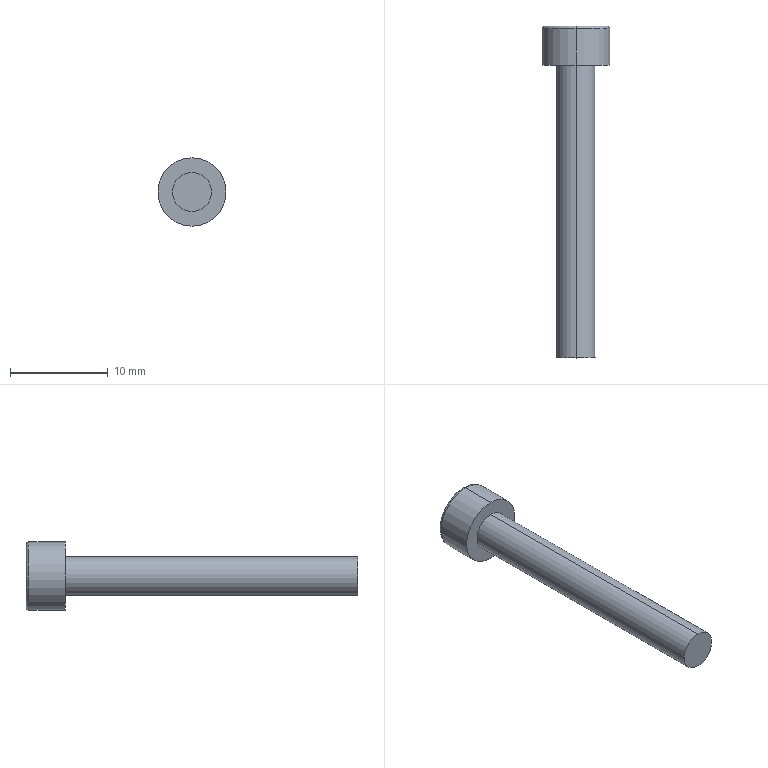Part | STEP file | M4 socket head cap screw simplified_M4X30 | 1 solid | 16 faces | box 7 x 34 x 7 mm | volume 513.868 mm3 | plane 10 | cylinder 4 | torus 2 | commonest cylinder face diameters 4 x2 7 x2
STEP:
#1=CARTESIAN_POINT('',(0.,0.,0.));
#2=DIRECTION('',(0.,0.,1.));
#3=DIRECTION('',(1.,0.,0.));
#4=AXIS2_PLACEMENT_3D('',#1,#2,#3);
#5=CARTESIAN_POINT('',(0.,0.,3.2));
#6=VERTEX_POINT('',#5);
#7=CARTESIAN_POINT('',(0.,0.,-3.2));
#8=VERTEX_POINT('',#7);
#9=CARTESIAN_POINT('',(0.,0.,0.));
#10=DIRECTION('',(0.,1.,0.));
#11=DIRECTION('',(0.,0.,-1.));
#12=AXIS2_PLACEMENT_3D('',#9,#10,#11);
#13=CIRCLE('',#12,3.2);
#14=CARTESIAN_POINT('',(0.,-0.3,0.));
#15=DIRECTION('',(0.,-1.,0.));
#16=DIRECTION('',(0.,0.,-1.));
#17=AXIS2_PLACEMENT_3D('',#14,#15,#16);
#18=TOROIDAL_SURFACE('',#17,3.2,0.3);
#19=CARTESIAN_POINT('',(6.283,4.712));
#20=DIRECTION('',(-1.,0.));
#21=VECTOR('',#20,1.);
#22=LINE('',#19,#21);
#23=(GEOMETRIC_REPRESENTATION_CONTEXT(2)PARAMETRIC_REPRESENTATION_CONTEXT()REPRESENTATION_CONTEXT('',''));
#24=DEFINITIONAL_REPRESENTATION('',(#22),#23);
#25=PCURVE('',#18,#24);
#26=CARTESIAN_POINT('',(0.,0.,0.));
#27=DIRECTION('',(0.,-1.,0.));
#28=DIRECTION('',(0.,0.,-1.));
#29=AXIS2_PLACEMENT_3D('',#26,#27,#28);
#30=PLANE('',#29);
#31=CARTESIAN_POINT('',(3.2,0.));
#32=CARTESIAN_POINT('',(3.2,-5.543));
#33=CARTESIAN_POINT('',(-1.6,-2.771));
#34=CARTESIAN_POINT('',(-6.4,0.));
#35=CARTESIAN_POINT('',(-1.6,2.771));
#36=CARTESIAN_POINT('',(3.2,5.543));
#37=CARTESIAN_POINT('',(3.2,0.));
#38=(BOUNDED_CURVE()B_SPLINE_CURVE(2,(#31,#32,#33,#34,#35,#36,#37),.UNSPECIFIED.,.T.,.F.)B_SPLINE_CURVE_WITH_KNOTS((1,2,2,2,2,1),(-2.094,0.,2.094,4.189,6.283,8.378),.UNSPECIFIED.)CURVE()GEOMETRIC_REPRESENTATION_ITEM()RATIONAL_B_SPLINE_CURVE((1.,0.5,1.,0.5,1.,0.5,1.))REPRESENTATION_ITEM(''));
#39=(GEOMETRIC_REPRESENTATION_CONTEXT(2)PARAMETRIC_REPRESENTATION_CONTEXT()REPRESENTATION_CONTEXT('',''));
#40=DEFINITIONAL_REPRESENTATION('',(#38),#39);
#41=PCURVE('',#30,#40);
#42=SURFACE_CURVE('',#13,(#25,#41),.PCURVE_S1.);
#43=EDGE_CURVE('',#6,#8,#42,.T.);
#44=ORIENTED_EDGE('',*,*,#43,.F.);
#45=CARTESIAN_POINT('',(0.,-0.3,3.5));
#46=VERTEX_POINT('',#45);
#47=CARTESIAN_POINT('',(0.,-0.3,3.2));
#48=DIRECTION('',(1.,0.,0.));
#49=DIRECTION('',(0.,0.,-1.));
#50=AXIS2_PLACEMENT_3D('',#47,#48,#49);
#51=CIRCLE('',#50,0.3);
#52=CARTESIAN_POINT('',(3.142,3.142));
#53=DIRECTION('',(0.,1.));
#54=VECTOR('',#53,1.);
#55=LINE('',#52,#54);
#56=(GEOMETRIC_REPRESENTATION_CONTEXT(2)PARAMETRIC_REPRESENTATION_CONTEXT()REPRESENTATION_CONTEXT('',''));
#57=DEFINITIONAL_REPRESENTATION('',(#55),#56);
#58=PCURVE('',#18,#57);
#59=CARTESIAN_POINT('',(0.,-0.3,0.));
#60=DIRECTION('',(0.,-1.,0.));
#61=DIRECTION('',(0.,0.,-1.));
#62=AXIS2_PLACEMENT_3D('',#59,#60,#61);
#63=TOROIDAL_SURFACE('',#62,3.2,0.3);
#64=CARTESIAN_POINT('',(3.142,3.142));
#65=DIRECTION('',(0.,1.));
#66=VECTOR('',#65,1.);
#67=LINE('',#64,#66);
#68=(GEOMETRIC_REPRESENTATION_CONTEXT(2)PARAMETRIC_REPRESENTATION_CONTEXT()REPRESENTATION_CONTEXT('',''));
#69=DEFINITIONAL_REPRESENTATION('',(#67),#68);
#70=PCURVE('',#63,#69);
#71=SURFACE_CURVE('',#51,(#58,#70),.PCURVE_S1.);
#72=EDGE_CURVE('',#6,#46,#71,.T.);
#73=ORIENTED_EDGE('',*,*,#72,.T.);
#74=CARTESIAN_POINT('',(0.,-0.3,-3.5));
#75=VERTEX_POINT('',#74);
#76=CARTESIAN_POINT('',(0.,-0.3,0.));
#77=DIRECTION('',(0.,-1.,0.));
#78=DIRECTION('',(0.,0.,-1.));
#79=AXIS2_PLACEMENT_3D('',#76,#77,#78);
#80=CIRCLE('',#79,3.5);
#81=CARTESIAN_POINT('',(0.,6.283));
#82=DIRECTION('',(1.,0.));
#83=VECTOR('',#82,1.);
#84=LINE('',#81,#83);
#85=(GEOMETRIC_REPRESENTATION_CONTEXT(2)PARAMETRIC_REPRESENTATION_CONTEXT()REPRESENTATION_CONTEXT('',''));
#86=DEFINITIONAL_REPRESENTATION('',(#84),#85);
#87=PCURVE('',#18,#86);
#88=CARTESIAN_POINT('',(0.,0.,0.));
#89=DIRECTION('',(0.,1.,0.));
#90=DIRECTION('',(0.,0.,1.));
#91=AXIS2_PLACEMENT_3D('',#88,#89,#90);
#92=CYLINDRICAL_SURFACE('',#91,3.5);
#93=CARTESIAN_POINT('',(3.142,-0.3));
#94=DIRECTION('',(-1.,0.));
#95=VECTOR('',#94,1.);
#96=LINE('',#93,#95);
#97=(GEOMETRIC_REPRESENTATION_CONTEXT(2)PARAMETRIC_REPRESENTATION_CONTEXT()REPRESENTATION_CONTEXT('',''));
#98=DEFINITIONAL_REPRESENTATION('',(#96),#97);
#99=PCURVE('',#92,#98);
#100=SURFACE_CURVE('',#80,(#87,#99),.PCURVE_S1.);
#101=EDGE_CURVE('',#75,#46,#100,.T.);
#102=ORIENTED_EDGE('',*,*,#101,.F.);
#103=CARTESIAN_POINT('',(0.,-0.3,-3.2));
#104=DIRECTION('',(-1.,0.,0.));
#105=DIRECTION('',(0.,0.,1.));
#106=AXIS2_PLACEMENT_3D('',#103,#104,#105);
#107=CIRCLE('',#106,0.3);
#108=CARTESIAN_POINT('',(0.,3.142));
#109=DIRECTION('',(0.,1.));
#110=VECTOR('',#109,1.);
#111=LINE('',#108,#110);
#112=(GEOMETRIC_REPRESENTATION_CONTEXT(2)PARAMETRIC_REPRESENTATION_CONTEXT()REPRESENTATION_CONTEXT('',''));
#113=DEFINITIONAL_REPRESENTATION('',(#111),#112);
#114=PCURVE('',#18,#113);
#115=CARTESIAN_POINT('',(6.283,3.142));
#116=DIRECTION('',(0.,1.));
#117=VECTOR('',#116,1.);
#118=LINE('',#115,#117);
#119=(GEOMETRIC_REPRESENTATION_CONTEXT(2)PARAMETRIC_REPRESENTATION_CONTEXT()REPRESENTATION_CONTEXT('',''));
#120=DEFINITIONAL_REPRESENTATION('',(#118),#119);
#121=PCURVE('',#63,#120);
#122=SURFACE_CURVE('',#107,(#114,#121),.PCURVE_S1.);
#123=EDGE_CURVE('',#8,#75,#122,.T.);
#124=ORIENTED_EDGE('',*,*,#123,.F.);
#125=EDGE_LOOP('',(#44,#73,#102,#124));
#126=FACE_BOUND('',#125,.T.);
#127=ADVANCED_FACE('',(#126),#18,.T.);
#128=CARTESIAN_POINT('',(0.,-34.,2.));
#129=VERTEX_POINT('',#128);
#130=CARTESIAN_POINT('',(0.,-34.,-2.));
#131=VERTEX_POINT('',#130);
#132=CARTESIAN_POINT('',(0.,-34.,0.));
#133=DIRECTION('',(0.,1.,0.));
#134=DIRECTION('',(0.,0.,1.));
#135=AXIS2_PLACEMENT_3D('',#132,#133,#134);
#136=CIRCLE('',#135,2.);
#137=CARTESIAN_POINT('',(0.,0.,0.));
#138=DIRECTION('',(0.,1.,0.));
#139=DIRECTION('',(0.,0.,1.));
#140=AXIS2_PLACEMENT_3D('',#137,#138,#139);
#141=CYLINDRICAL_SURFACE('',#140,2.);
#142=CARTESIAN_POINT('',(0.,-34.));
#143=DIRECTION('',(1.,0.));
#144=VECTOR('',#143,1.);
#145=LINE('',#142,#144);
#146=(GEOMETRIC_REPRESENTATION_CONTEXT(2)PARAMETRIC_REPRESENTATION_CONTEXT()REPRESENTATION_CONTEXT('',''));
#147=DEFINITIONAL_REPRESENTATION('',(#145),#146);
#148=PCURVE('',#141,#147);
#149=CARTESIAN_POINT('',(2.,-34.,0.));
#150=DIRECTION('',(0.,1.,0.));
#151=DIRECTION('',(0.,0.,1.));
#152=AXIS2_PLACEMENT_3D('',#149,#150,#151);
#153=PLANE('',#152);
#154=CARTESIAN_POINT('',(0.,-2.));
#155=DIRECTION('',(1.,0.));
#156=AXIS2_PLACEMENT_2D('',#154,#155);
#157=CIRCLE('',#156,2.);
#158=(GEOMETRIC_REPRESENTATION_CONTEXT(2)PARAMETRIC_REPRESENTATION_CONTEXT()REPRESENTATION_CONTEXT('',''));
#159=DEFINITIONAL_REPRESENTATION('',(#157),#158);
#160=PCURVE('',#153,#159);
#161=SURFACE_CURVE('',#136,(#148,#160),.PCURVE_S1.);
#162=EDGE_CURVE('',#129,#131,#161,.T.);
#163=ORIENTED_EDGE('',*,*,#162,.T.);
#164=CARTESIAN_POINT('',(0.,-4.,-2.));
#165=VERTEX_POINT('',#164);
#166=CARTESIAN_POINT('',(0.,0.,-2.));
#167=DIRECTION('',(0.,1.,0.));
#168=VECTOR('',#167,1.);
#169=LINE('',#166,#168);
#170=CARTESIAN_POINT('',(3.142,0.));
#171=DIRECTION('',(0.,1.));
#172=VECTOR('',#171,1.);
#173=LINE('',#170,#172);
#174=(GEOMETRIC_REPRESENTATION_CONTEXT(2)PARAMETRIC_REPRESENTATION_CONTEXT()REPRESENTATION_CONTEXT('',''));
#175=DEFINITIONAL_REPRESENTATION('',(#173),#174);
#176=PCURVE('',#141,#175);
#177=CARTESIAN_POINT('',(0.,0.,0.));
#178=DIRECTION('',(0.,1.,0.));
#179=DIRECTION('',(0.,0.,1.));
#180=AXIS2_PLACEMENT_3D('',#177,#178,#179);
#181=CYLINDRICAL_SURFACE('',#180,2.);
#182=CARTESIAN_POINT('',(3.142,0.));
#183=DIRECTION('',(0.,1.));
#184=VECTOR('',#183,1.);
#185=LINE('',#182,#184);
#186=(GEOMETRIC_REPRESENTATION_CONTEXT(2)PARAMETRIC_REPRESENTATION_CONTEXT()REPRESENTATION_CONTEXT('',''));
#187=DEFINITIONAL_REPRESENTATION('',(#185),#186);
#188=PCURVE('',#181,#187);
#189=SURFACE_CURVE('',#169,(#176,#188),.PCURVE_S1.);
#190=EDGE_CURVE('',#131,#165,#189,.T.);
#191=ORIENTED_EDGE('',*,*,#190,.T.);
#192=CARTESIAN_POINT('',(0.,-4.,2.));
#193=VERTEX_POINT('',#192);
#194=CARTESIAN_POINT('',(0.,-4.,0.));
#195=DIRECTION('',(0.,1.,0.));
#196=DIRECTION('',(0.,0.,1.));
#197=AXIS2_PLACEMENT_3D('',#194,#195,#196);
#198=CIRCLE('',#197,2.);
#199=CARTESIAN_POINT('',(0.,-4.));
#200=DIRECTION('',(1.,0.));
#201=VECTOR('',#200,1.);
#202=LINE('',#199,#201);
#203=(GEOMETRIC_REPRESENTATION_CONTEXT(2)PARAMETRIC_REPRESENTATION_CONTEXT()REPRESENTATION_CONTEXT('',''));
#204=DEFINITIONAL_REPRESENTATION('',(#202),#203);
#205=PCURVE('',#141,#204);
#206=CARTESIAN_POINT('',(3.5,-4.,0.));
#207=DIRECTION('',(0.,1.,0.));
#208=DIRECTION('',(0.,0.,1.));
#209=AXIS2_PLACEMENT_3D('',#206,#207,#208);
#210=PLANE('',#209);
#211=CARTESIAN_POINT('',(0.,-3.5));
#212=DIRECTION('',(1.,0.));
#213=AXIS2_PLACEMENT_2D('',#211,#212);
#214=CIRCLE('',#213,2.);
#215=(GEOMETRIC_REPRESENTATION_CONTEXT(2)PARAMETRIC_REPRESENTATION_CONTEXT()REPRESENTATION_CONTEXT('',''));
#216=DEFINITIONAL_REPRESENTATION('',(#214),#215);
#217=PCURVE('',#210,#216);
#218=SURFACE_CURVE('',#198,(#205,#217),.PCURVE_S1.);
#219=EDGE_CURVE('',#193,#165,#218,.T.);
#220=ORIENTED_EDGE('',*,*,#219,.F.);
#221=CARTESIAN_POINT('',(0.,0.,2.));
#222=DIRECTION('',(0.,1.,0.));
#223=VECTOR('',#222,1.);
#224=LINE('',#221,#223);
#225=CARTESIAN_POINT('',(0.,0.));
#226=DIRECTION('',(0.,1.));
#227=VECTOR('',#226,1.);
#228=LINE('',#225,#227);
#229=(GEOMETRIC_REPRESENTATION_CONTEXT(2)PARAMETRIC_REPRESENTATION_CONTEXT()REPRESENTATION_CONTEXT('',''));
#230=DEFINITIONAL_REPRESENTATION('',(#228),#229);
#231=PCURVE('',#141,#230);
#232=CARTESIAN_POINT('',(6.283,0.));
#233=DIRECTION('',(0.,1.));
#234=VECTOR('',#233,1.);
#235=LINE('',#232,#234);
#236=(GEOMETRIC_REPRESENTATION_CONTEXT(2)PARAMETRIC_REPRESENTATION_CONTEXT()REPRESENTATION_CONTEXT('',''));
#237=DEFINITIONAL_REPRESENTATION('',(#235),#236);
#238=PCURVE('',#181,#237);
#239=SURFACE_CURVE('',#224,(#231,#238),.PCURVE_S1.);
#240=EDGE_CURVE('',#129,#193,#239,.T.);
#241=ORIENTED_EDGE('',*,*,#240,.F.);
#242=EDGE_LOOP('',(#163,#191,#220,#241));
#243=FACE_BOUND('',#242,.T.);
#244=ADVANCED_FACE('',(#243),#141,.T.);
#245=CARTESIAN_POINT('',(0.,-4.,3.5));
#246=VERTEX_POINT('',#245);
#247=CARTESIAN_POINT('',(0.,-4.,-3.5));
#248=VERTEX_POINT('',#247);
#249=CARTESIAN_POINT('',(0.,-4.,0.));
#250=DIRECTION('',(0.,1.,0.));
#251=DIRECTION('',(0.,0.,1.));
#252=AXIS2_PLACEMENT_3D('',#249,#250,#251);
#253=CIRCLE('',#252,3.5);
#254=CARTESIAN_POINT('',(0.,-4.));
#255=DIRECTION('',(1.,0.));
#256=VECTOR('',#255,1.);
#257=LINE('',#254,#256);
#258=(GEOMETRIC_REPRESENTATION_CONTEXT(2)PARAMETRIC_REPRESENTATION_CONTEXT()REPRESENTATION_CONTEXT('',''));
#259=DEFINITIONAL_REPRESENTATION('',(#257),#258);
#260=PCURVE('',#92,#259);
#261=CARTESIAN_POINT('',(0.,-3.5));
#262=DIRECTION('',(1.,0.));
#263=AXIS2_PLACEMENT_2D('',#261,#262);
#264=CIRCLE('',#263,3.5);
#265=(GEOMETRIC_REPRESENTATION_CONTEXT(2)PARAMETRIC_REPRESENTATION_CONTEXT()REPRESENTATION_CONTEXT('',''));
#266=DEFINITIONAL_REPRESENTATION('',(#264),#265);
#267=PCURVE('',#210,#266);
#268=SURFACE_CURVE('',#253,(#260,#267),.PCURVE_S1.);
#269=EDGE_CURVE('',#246,#248,#268,.T.);
#270=ORIENTED_EDGE('',*,*,#269,.T.);
#271=CARTESIAN_POINT('',(0.,0.,-3.5));
#272=DIRECTION('',(0.,1.,0.));
#273=VECTOR('',#272,1.);
#274=LINE('',#271,#273);
#275=CARTESIAN_POINT('',(3.142,0.));
#276=DIRECTION('',(0.,1.));
#277=VECTOR('',#276,1.);
#278=LINE('',#275,#277);
#279=(GEOMETRIC_REPRESENTATION_CONTEXT(2)PARAMETRIC_REPRESENTATION_CONTEXT()REPRESENTATION_CONTEXT('',''));
#280=DEFINITIONAL_REPRESENTATION('',(#278),#279);
#281=PCURVE('',#92,#280);
#282=CARTESIAN_POINT('',(0.,0.,0.));
#283=DIRECTION('',(0.,1.,0.));
#284=DIRECTION('',(0.,0.,1.));
#285=AXIS2_PLACEMENT_3D('',#282,#283,#284);
#286=CYLINDRICAL_SURFACE('',#285,3.5);
#287=CARTESIAN_POINT('',(3.142,0.));
#288=DIRECTION('',(0.,1.));
#289=VECTOR('',#288,1.);
#290=LINE('',#287,#289);
#291=(GEOMETRIC_REPRESENTATION_CONTEXT(2)PARAMETRIC_REPRESENTATION_CONTEXT()REPRESENTATION_CONTEXT('',''));
#292=DEFINITIONAL_REPRESENTATION('',(#290),#291);
#293=PCURVE('',#286,#292);
#294=SURFACE_CURVE('',#274,(#281,#293),.PCURVE_S1.);
#295=EDGE_CURVE('',#248,#75,#294,.T.);
#296=ORIENTED_EDGE('',*,*,#295,.T.);
#297=ORIENTED_EDGE('',*,*,#101,.T.);
#298=CARTESIAN_POINT('',(0.,0.,3.5));
#299=DIRECTION('',(0.,1.,0.));
#300=VECTOR('',#299,1.);
#301=LINE('',#298,#300);
#302=CARTESIAN_POINT('',(0.,0.));
#303=DIRECTION('',(0.,1.));
#304=VECTOR('',#303,1.);
#305=LINE('',#302,#304);
#306=(GEOMETRIC_REPRESENTATION_CONTEXT(2)PARAMETRIC_REPRESENTATION_CONTEXT()REPRESENTATION_CONTEXT('',''));
#307=DEFINITIONAL_REPRESENTATION('',(#305),#306);
#308=PCURVE('',#92,#307);
#309=CARTESIAN_POINT('',(6.283,0.));
#310=DIRECTION('',(0.,1.));
#311=VECTOR('',#310,1.);
#312=LINE('',#309,#311);
#313=(GEOMETRIC_REPRESENTATION_CONTEXT(2)PARAMETRIC_REPRESENTATION_CONTEXT()REPRESENTATION_CONTEXT('',''));
#314=DEFINITIONAL_REPRESENTATION('',(#312),#313);
#315=PCURVE('',#286,#314);
#316=SURFACE_CURVE('',#301,(#308,#315),.PCURVE_S1.);
#317=EDGE_CURVE('',#246,#46,#316,.T.);
#318=ORIENTED_EDGE('',*,*,#317,.F.);
#319=EDGE_LOOP('',(#270,#296,#297,#318));
#320=FACE_BOUND('',#319,.T.);
#321=ADVANCED_FACE('',(#320),#92,.T.);
#322=CARTESIAN_POINT('',(0.,0.,0.));
#323=DIRECTION('',(0.,1.,0.));
#324=DIRECTION('',(0.,0.,-1.));
#325=AXIS2_PLACEMENT_3D('',#322,#323,#324);
#326=CIRCLE('',#325,3.2);
#327=CARTESIAN_POINT('',(3.2,0.));
#328=CARTESIAN_POINT('',(3.2,-5.543));
#329=CARTESIAN_POINT('',(-1.6,-2.771));
#330=CARTESIAN_POINT('',(-6.4,0.));
#331=CARTESIAN_POINT('',(-1.6,2.771));
#332=CARTESIAN_POINT('',(3.2,5.543));
#333=CARTESIAN_POINT('',(3.2,0.));
#334=(BOUNDED_CURVE()B_SPLINE_CURVE(2,(#327,#328,#329,#330,#331,#332,#333),.UNSPECIFIED.,.T.,.F.)B_SPLINE_CURVE_WITH_KNOTS((1,2,2,2,2,1),(-2.094,0.,2.094,4.189,6.283,8.378),.UNSPECIFIED.)CURVE()GEOMETRIC_REPRESENTATION_ITEM()RATIONAL_B_SPLINE_CURVE((1.,0.5,1.,0.5,1.,0.5,1.))REPRESENTATION_ITEM(''));
#335=(GEOMETRIC_REPRESENTATION_CONTEXT(2)PARAMETRIC_REPRESENTATION_CONTEXT()REPRESENTATION_CONTEXT('',''));
#336=DEFINITIONAL_REPRESENTATION('',(#334),#335);
#337=PCURVE('',#30,#336);
#338=CARTESIAN_POINT('',(6.283,4.712));
#339=DIRECTION('',(-1.,0.));
#340=VECTOR('',#339,1.);
#341=LINE('',#338,#340);
#342=(GEOMETRIC_REPRESENTATION_CONTEXT(2)PARAMETRIC_REPRESENTATION_CONTEXT()REPRESENTATION_CONTEXT('',''));
#343=DEFINITIONAL_REPRESENTATION('',(#341),#342);
#344=PCURVE('',#63,#343);
#345=SURFACE_CURVE('',#326,(#337,#344),.PCURVE_S1.);
#346=EDGE_CURVE('',#8,#6,#345,.T.);
#347=ORIENTED_EDGE('',*,*,#346,.T.);
#348=ORIENTED_EDGE('',*,*,#43,.T.);
#349=EDGE_LOOP('',(#347,#348));
#350=FACE_BOUND('',#349,.T.);
#351=CARTESIAN_POINT('',(-1.79,0.,0.));
#352=VERTEX_POINT('',#351);
#353=CARTESIAN_POINT('',(-0.8949,0.,1.55));
#354=VERTEX_POINT('',#353);
#355=CARTESIAN_POINT('',(-1.79,0.,0.));
#356=DIRECTION('',(0.5,0.,0.866));
#357=VECTOR('',#356,1.);
#358=LINE('',#355,#357);
#359=CARTESIAN_POINT('',(0.,-1.79));
#360=DIRECTION('',(-0.866,0.5));
#361=VECTOR('',#360,1.);
#362=LINE('',#359,#361);
#363=(GEOMETRIC_REPRESENTATION_CONTEXT(2)PARAMETRIC_REPRESENTATION_CONTEXT()REPRESENTATION_CONTEXT('',''));
#364=DEFINITIONAL_REPRESENTATION('',(#362),#363);
#365=PCURVE('',#30,#364);
#366=CARTESIAN_POINT('',(-1.79,-2.,0.));
#367=DIRECTION('',(-0.866,0.,0.5));
#368=DIRECTION('',(0.5,0.,0.866));
#369=AXIS2_PLACEMENT_3D('',#366,#367,#368);
#370=PLANE('',#369);
#371=CARTESIAN_POINT('',(0.,2.));
#372=DIRECTION('',(1.,0.));
#373=VECTOR('',#372,1.);
#374=LINE('',#371,#373);
#375=(GEOMETRIC_REPRESENTATION_CONTEXT(2)PARAMETRIC_REPRESENTATION_CONTEXT()REPRESENTATION_CONTEXT('',''));
#376=DEFINITIONAL_REPRESENTATION('',(#374),#375);
#377=PCURVE('',#370,#376);
#378=SURFACE_CURVE('',#358,(#365,#377),.PCURVE_S1.);
#379=EDGE_CURVE('',#352,#354,#378,.T.);
#380=ORIENTED_EDGE('',*,*,#379,.F.);
#381=CARTESIAN_POINT('',(-0.8949,0.,-1.55));
#382=VERTEX_POINT('',#381);
#383=CARTESIAN_POINT('',(-0.8949,0.,-1.55));
#384=DIRECTION('',(-0.5,0.,0.866));
#385=VECTOR('',#384,1.);
#386=LINE('',#383,#385);
#387=CARTESIAN_POINT('',(1.55,-0.8949));
#388=DIRECTION('',(-0.866,-0.5));
#389=VECTOR('',#388,1.);
#390=LINE('',#387,#389);
#391=(GEOMETRIC_REPRESENTATION_CONTEXT(2)PARAMETRIC_REPRESENTATION_CONTEXT()REPRESENTATION_CONTEXT('',''));
#392=DEFINITIONAL_REPRESENTATION('',(#390),#391);
#393=PCURVE('',#30,#392);
#394=CARTESIAN_POINT('',(-0.8949,-2.,-1.55));
#395=DIRECTION('',(-0.866,0.,-0.5));
#396=DIRECTION('',(-0.5,0.,0.866));
#397=AXIS2_PLACEMENT_3D('',#394,#395,#396);
#398=PLANE('',#397);
#399=CARTESIAN_POINT('',(0.,2.));
#400=DIRECTION('',(1.,0.));
#401=VECTOR('',#400,1.);
#402=LINE('',#399,#401);
#403=(GEOMETRIC_REPRESENTATION_CONTEXT(2)PARAMETRIC_REPRESENTATION_CONTEXT()REPRESENTATION_CONTEXT('',''));
#404=DEFINITIONAL_REPRESENTATION('',(#402),#403);
#405=PCURVE('',#398,#404);
#406=SURFACE_CURVE('',#386,(#393,#405),.PCURVE_S1.);
#407=EDGE_CURVE('',#382,#352,#406,.T.);
#408=ORIENTED_EDGE('',*,*,#407,.F.);
#409=CARTESIAN_POINT('',(0.8949,0.,-1.55));
#410=VERTEX_POINT('',#409);
#411=CARTESIAN_POINT('',(0.8949,0.,-1.55));
#412=DIRECTION('',(-1.,0.,0.));
#413=VECTOR('',#412,1.);
#414=LINE('',#411,#413);
#415=CARTESIAN_POINT('',(1.55,0.8949));
#416=DIRECTION('',(0.,-1.));
#417=VECTOR('',#416,1.);
#418=LINE('',#415,#417);
#419=(GEOMETRIC_REPRESENTATION_CONTEXT(2)PARAMETRIC_REPRESENTATION_CONTEXT()REPRESENTATION_CONTEXT('',''));
#420=DEFINITIONAL_REPRESENTATION('',(#418),#419);
#421=PCURVE('',#30,#420);
#422=CARTESIAN_POINT('',(0.8949,-2.,-1.55));
#423=DIRECTION('',(0.,0.,-1.));
#424=DIRECTION('',(-1.,0.,0.));
#425=AXIS2_PLACEMENT_3D('',#422,#423,#424);
#426=PLANE('',#425);
#427=CARTESIAN_POINT('',(0.,2.));
#428=DIRECTION('',(1.,0.));
#429=VECTOR('',#428,1.);
#430=LINE('',#427,#429);
#431=(GEOMETRIC_REPRESENTATION_CONTEXT(2)PARAMETRIC_REPRESENTATION_CONTEXT()REPRESENTATION_CONTEXT('',''));
#432=DEFINITIONAL_REPRESENTATION('',(#430),#431);
#433=PCURVE('',#426,#432);
#434=SURFACE_CURVE('',#414,(#421,#433),.PCURVE_S1.);
#435=EDGE_CURVE('',#410,#382,#434,.T.);
#436=ORIENTED_EDGE('',*,*,#435,.F.);
#437=CARTESIAN_POINT('',(1.79,0.,0.));
#438=VERTEX_POINT('',#437);
#439=CARTESIAN_POINT('',(1.79,0.,0.));
#440=DIRECTION('',(-0.5,0.,-0.866));
#441=VECTOR('',#440,1.);
#442=LINE('',#439,#441);
#443=CARTESIAN_POINT('',(0.,1.79));
#444=DIRECTION('',(0.866,-0.5));
#445=VECTOR('',#444,1.);
#446=LINE('',#443,#445);
#447=(GEOMETRIC_REPRESENTATION_CONTEXT(2)PARAMETRIC_REPRESENTATION_CONTEXT()REPRESENTATION_CONTEXT('',''));
#448=DEFINITIONAL_REPRESENTATION('',(#446),#447);
#449=PCURVE('',#30,#448);
#450=CARTESIAN_POINT('',(1.79,-2.,0.));
#451=DIRECTION('',(0.866,0.,-0.5));
#452=DIRECTION('',(-0.5,0.,-0.866));
#453=AXIS2_PLACEMENT_3D('',#450,#451,#452);
#454=PLANE('',#453);
#455=CARTESIAN_POINT('',(0.,2.));
#456=DIRECTION('',(1.,0.));
#457=VECTOR('',#456,1.);
#458=LINE('',#455,#457);
#459=(GEOMETRIC_REPRESENTATION_CONTEXT(2)PARAMETRIC_REPRESENTATION_CONTEXT()REPRESENTATION_CONTEXT('',''));
#460=DEFINITIONAL_REPRESENTATION('',(#458),#459);
#461=PCURVE('',#454,#460);
#462=SURFACE_CURVE('',#442,(#449,#461),.PCURVE_S1.);
#463=EDGE_CURVE('',#438,#410,#462,.T.);
#464=ORIENTED_EDGE('',*,*,#463,.F.);
#465=CARTESIAN_POINT('',(0.8949,0.,1.55));
#466=VERTEX_POINT('',#465);
#467=CARTESIAN_POINT('',(0.8949,0.,1.55));
#468=DIRECTION('',(0.5,0.,-0.866));
#469=VECTOR('',#468,1.);
#470=LINE('',#467,#469);
#471=CARTESIAN_POINT('',(-1.55,0.8949));
#472=DIRECTION('',(0.866,0.5));
#473=VECTOR('',#472,1.);
#474=LINE('',#471,#473);
#475=(GEOMETRIC_REPRESENTATION_CONTEXT(2)PARAMETRIC_REPRESENTATION_CONTEXT()REPRESENTATION_CONTEXT('',''));
#476=DEFINITIONAL_REPRESENTATION('',(#474),#475);
#477=PCURVE('',#30,#476);
#478=CARTESIAN_POINT('',(0.8949,-2.,1.55));
#479=DIRECTION('',(0.866,0.,0.5));
#480=DIRECTION('',(0.5,0.,-0.866));
#481=AXIS2_PLACEMENT_3D('',#478,#479,#480);
#482=PLANE('',#481);
#483=CARTESIAN_POINT('',(0.,2.));
#484=DIRECTION('',(1.,0.));
#485=VECTOR('',#484,1.);
#486=LINE('',#483,#485);
#487=(GEOMETRIC_REPRESENTATION_CONTEXT(2)PARAMETRIC_REPRESENTATION_CONTEXT()REPRESENTATION_CONTEXT('',''));
#488=DEFINITIONAL_REPRESENTATION('',(#486),#487);
#489=PCURVE('',#482,#488);
#490=SURFACE_CURVE('',#470,(#477,#489),.PCURVE_S1.);
#491=EDGE_CURVE('',#466,#438,#490,.T.);
#492=ORIENTED_EDGE('',*,*,#491,.F.);
#493=CARTESIAN_POINT('',(-0.8949,0.,1.55));
#494=DIRECTION('',(1.,0.,0.));
#495=VECTOR('',#494,1.);
#496=LINE('',#493,#495);
#497=CARTESIAN_POINT('',(-1.55,-0.8949));
#498=DIRECTION('',(0.,1.));
#499=VECTOR('',#498,1.);
#500=LINE('',#497,#499);
#501=(GEOMETRIC_REPRESENTATION_CONTEXT(2)PARAMETRIC_REPRESENTATION_CONTEXT()REPRESENTATION_CONTEXT('',''));
#502=DEFINITIONAL_REPRESENTATION('',(#500),#501);
#503=PCURVE('',#30,#502);
#504=CARTESIAN_POINT('',(-0.8949,-2.,1.55));
#505=DIRECTION('',(0.,0.,1.));
#506=DIRECTION('',(1.,0.,0.));
#507=AXIS2_PLACEMENT_3D('',#504,#505,#506);
#508=PLANE('',#507);
#509=CARTESIAN_POINT('',(0.,2.));
#510=DIRECTION('',(1.,0.));
#511=VECTOR('',#510,1.);
#512=LINE('',#509,#511);
#513=(GEOMETRIC_REPRESENTATION_CONTEXT(2)PARAMETRIC_REPRESENTATION_CONTEXT()REPRESENTATION_CONTEXT('',''));
#514=DEFINITIONAL_REPRESENTATION('',(#512),#513);
#515=PCURVE('',#508,#514);
#516=SURFACE_CURVE('',#496,(#503,#515),.PCURVE_S1.);
#517=EDGE_CURVE('',#354,#466,#516,.T.);
#518=ORIENTED_EDGE('',*,*,#517,.F.);
#519=EDGE_LOOP('',(#380,#408,#436,#464,#492,#518));
#520=FACE_BOUND('',#519,.T.);
#521=ADVANCED_FACE('',(#350,#520),#30,.F.);
#522=ORIENTED_EDGE('',*,*,#295,.F.);
#523=CARTESIAN_POINT('',(0.,-4.,0.));
#524=DIRECTION('',(0.,1.,0.));
#525=DIRECTION('',(0.,0.,1.));
#526=AXIS2_PLACEMENT_3D('',#523,#524,#525);
#527=CIRCLE('',#526,3.5);
#528=CARTESIAN_POINT('',(0.,-4.));
#529=DIRECTION('',(1.,0.));
#530=VECTOR('',#529,1.);
#531=LINE('',#528,#530);
#532=(GEOMETRIC_REPRESENTATION_CONTEXT(2)PARAMETRIC_REPRESENTATION_CONTEXT()REPRESENTATION_CONTEXT('',''));
#533=DEFINITIONAL_REPRESENTATION('',(#531),#532);
#534=PCURVE('',#286,#533);
#535=CARTESIAN_POINT('',(0.,-3.5));
#536=DIRECTION('',(1.,0.));
#537=AXIS2_PLACEMENT_2D('',#535,#536);
#538=CIRCLE('',#537,3.5);
#539=(GEOMETRIC_REPRESENTATION_CONTEXT(2)PARAMETRIC_REPRESENTATION_CONTEXT()REPRESENTATION_CONTEXT('',''));
#540=DEFINITIONAL_REPRESENTATION('',(#538),#539);
#541=PCURVE('',#210,#540);
#542=SURFACE_CURVE('',#527,(#534,#541),.PCURVE_S1.);
#543=EDGE_CURVE('',#248,#246,#542,.T.);
#544=ORIENTED_EDGE('',*,*,#543,.T.);
#545=ORIENTED_EDGE('',*,*,#317,.T.);
#546=CARTESIAN_POINT('',(0.,-0.3,0.));
#547=DIRECTION('',(0.,-1.,0.));
#548=DIRECTION('',(0.,0.,-1.));
#549=AXIS2_PLACEMENT_3D('',#546,#547,#548);
#550=CIRCLE('',#549,3.5);
#551=CARTESIAN_POINT('',(9.425,-0.3));
#552=DIRECTION('',(-1.,0.));
#553=VECTOR('',#552,1.);
#554=LINE('',#551,#553);
#555=(GEOMETRIC_REPRESENTATION_CONTEXT(2)PARAMETRIC_REPRESENTATION_CONTEXT()REPRESENTATION_CONTEXT('',''));
#556=DEFINITIONAL_REPRESENTATION('',(#554),#555);
#557=PCURVE('',#286,#556);
#558=CARTESIAN_POINT('',(0.,6.283));
#559=DIRECTION('',(1.,0.));
#560=VECTOR('',#559,1.);
#561=LINE('',#558,#560);
#562=(GEOMETRIC_REPRESENTATION_CONTEXT(2)PARAMETRIC_REPRESENTATION_CONTEXT()REPRESENTATION_CONTEXT('',''));
#563=DEFINITIONAL_REPRESENTATION('',(#561),#562);
#564=PCURVE('',#63,#563);
#565=SURFACE_CURVE('',#550,(#557,#564),.PCURVE_S1.);
#566=EDGE_CURVE('',#46,#75,#565,.T.);
#567=ORIENTED_EDGE('',*,*,#566,.T.);
#568=EDGE_LOOP('',(#522,#544,#545,#567));
#569=FACE_BOUND('',#568,.T.);
#570=ADVANCED_FACE('',(#569),#286,.T.);
#571=ORIENTED_EDGE('',*,*,#269,.F.);
#572=ORIENTED_EDGE('',*,*,#543,.F.);
#573=EDGE_LOOP('',(#571,#572));
#574=FACE_BOUND('',#573,.T.);
#575=ORIENTED_EDGE('',*,*,#219,.T.);
#576=CARTESIAN_POINT('',(0.,-4.,0.));
#577=DIRECTION('',(0.,1.,0.));
#578=DIRECTION('',(0.,0.,1.));
#579=AXIS2_PLACEMENT_3D('',#576,#577,#578);
#580=CIRCLE('',#579,2.);
#581=CARTESIAN_POINT('',(0.,-3.5));
#582=DIRECTION('',(1.,0.));
#583=AXIS2_PLACEMENT_2D('',#581,#582);
#584=CIRCLE('',#583,2.);
#585=(GEOMETRIC_REPRESENTATION_CONTEXT(2)PARAMETRIC_REPRESENTATION_CONTEXT()REPRESENTATION_CONTEXT('',''));
#586=DEFINITIONAL_REPRESENTATION('',(#584),#585);
#587=PCURVE('',#210,#586);
#588=CARTESIAN_POINT('',(0.,-4.));
#589=DIRECTION('',(1.,0.));
#590=VECTOR('',#589,1.);
#591=LINE('',#588,#590);
#592=(GEOMETRIC_REPRESENTATION_CONTEXT(2)PARAMETRIC_REPRESENTATION_CONTEXT()REPRESENTATION_CONTEXT('',''));
#593=DEFINITIONAL_REPRESENTATION('',(#591),#592);
#594=PCURVE('',#181,#593);
#595=SURFACE_CURVE('',#580,(#587,#594),.PCURVE_S1.);
#596=EDGE_CURVE('',#165,#193,#595,.T.);
#597=ORIENTED_EDGE('',*,*,#596,.T.);
#598=EDGE_LOOP('',(#575,#597));
#599=FACE_BOUND('',#598,.T.);
#600=ADVANCED_FACE('',(#574,#599),#210,.F.);
#601=ORIENTED_EDGE('',*,*,#190,.F.);
#602=CARTESIAN_POINT('',(0.,-34.,0.));
#603=DIRECTION('',(0.,1.,0.));
#604=DIRECTION('',(0.,0.,1.));
#605=AXIS2_PLACEMENT_3D('',#602,#603,#604);
#606=CIRCLE('',#605,2.);
#607=CARTESIAN_POINT('',(0.,-34.));
#608=DIRECTION('',(1.,0.));
#609=VECTOR('',#608,1.);
#610=LINE('',#607,#609);
#611=(GEOMETRIC_REPRESENTATION_CONTEXT(2)PARAMETRIC_REPRESENTATION_CONTEXT()REPRESENTATION_CONTEXT('',''));
#612=DEFINITIONAL_REPRESENTATION('',(#610),#611);
#613=PCURVE('',#181,#612);
#614=CARTESIAN_POINT('',(0.,-2.));
#615=DIRECTION('',(1.,0.));
#616=AXIS2_PLACEMENT_2D('',#614,#615);
#617=CIRCLE('',#616,2.);
#618=(GEOMETRIC_REPRESENTATION_CONTEXT(2)PARAMETRIC_REPRESENTATION_CONTEXT()REPRESENTATION_CONTEXT('',''));
#619=DEFINITIONAL_REPRESENTATION('',(#617),#618);
#620=PCURVE('',#153,#619);
#621=SURFACE_CURVE('',#606,(#613,#620),.PCURVE_S1.);
#622=EDGE_CURVE('',#131,#129,#621,.T.);
#623=ORIENTED_EDGE('',*,*,#622,.T.);
#624=ORIENTED_EDGE('',*,*,#240,.T.);
#625=ORIENTED_EDGE('',*,*,#596,.F.);
#626=EDGE_LOOP('',(#601,#623,#624,#625));
#627=FACE_BOUND('',#626,.T.);
#628=ADVANCED_FACE('',(#627),#181,.T.);
#629=ORIENTED_EDGE('',*,*,#162,.F.);
#630=ORIENTED_EDGE('',*,*,#622,.F.);
#631=EDGE_LOOP('',(#629,#630));
#632=FACE_BOUND('',#631,.T.);
#633=ADVANCED_FACE('',(#632),#153,.F.);
#634=ORIENTED_EDGE('',*,*,#407,.T.);
#635=CARTESIAN_POINT('',(-1.79,-2.,0.));
#636=VERTEX_POINT('',#635);
#637=CARTESIAN_POINT('',(-1.79,-2.,0.));
#638=DIRECTION('',(0.,1.,0.));
#639=VECTOR('',#638,1.);
#640=LINE('',#637,#639);
#641=CARTESIAN_POINT('',(1.79,0.));
#642=DIRECTION('',(0.,1.));
#643=VECTOR('',#642,1.);
#644=LINE('',#641,#643);
#645=(GEOMETRIC_REPRESENTATION_CONTEXT(2)PARAMETRIC_REPRESENTATION_CONTEXT()REPRESENTATION_CONTEXT('',''));
#646=DEFINITIONAL_REPRESENTATION('',(#644),#645);
#647=PCURVE('',#398,#646);
#648=CARTESIAN_POINT('',(0.,0.));
#649=DIRECTION('',(0.,1.));
#650=VECTOR('',#649,1.);
#651=LINE('',#648,#650);
#652=(GEOMETRIC_REPRESENTATION_CONTEXT(2)PARAMETRIC_REPRESENTATION_CONTEXT()REPRESENTATION_CONTEXT('',''));
#653=DEFINITIONAL_REPRESENTATION('',(#651),#652);
#654=PCURVE('',#370,#653);
#655=SURFACE_CURVE('',#640,(#647,#654),.PCURVE_S1.);
#656=EDGE_CURVE('',#636,#352,#655,.T.);
#657=ORIENTED_EDGE('',*,*,#656,.F.);
#658=CARTESIAN_POINT('',(-0.8949,-2.,-1.55));
#659=VERTEX_POINT('',#658);
#660=CARTESIAN_POINT('',(-0.8949,-2.,-1.55));
#661=DIRECTION('',(-0.5,0.,0.866));
#662=VECTOR('',#661,1.);
#663=LINE('',#660,#662);
#664=CARTESIAN_POINT('',(0.,0.));
#665=DIRECTION('',(1.,0.));
#666=VECTOR('',#665,1.);
#667=LINE('',#664,#666);
#668=(GEOMETRIC_REPRESENTATION_CONTEXT(2)PARAMETRIC_REPRESENTATION_CONTEXT()REPRESENTATION_CONTEXT('',''));
#669=DEFINITIONAL_REPRESENTATION('',(#667),#668);
#670=PCURVE('',#398,#669);
#671=CARTESIAN_POINT('',(-1.79,-2.,0.));
#672=DIRECTION('',(0.,1.,0.));
#673=DIRECTION('',(0.,0.,1.));
#674=AXIS2_PLACEMENT_3D('',#671,#672,#673);
#675=PLANE('',#674);
#676=CARTESIAN_POINT('',(-1.55,0.8949));
#677=DIRECTION('',(0.866,-0.5));
#678=VECTOR('',#677,1.);
#679=LINE('',#676,#678);
#680=(GEOMETRIC_REPRESENTATION_CONTEXT(2)PARAMETRIC_REPRESENTATION_CONTEXT()REPRESENTATION_CONTEXT('',''));
#681=DEFINITIONAL_REPRESENTATION('',(#679),#680);
#682=PCURVE('',#675,#681);
#683=SURFACE_CURVE('',#663,(#670,#682),.PCURVE_S1.);
#684=EDGE_CURVE('',#659,#636,#683,.T.);
#685=ORIENTED_EDGE('',*,*,#684,.F.);
#686=CARTESIAN_POINT('',(-0.8949,-2.,-1.55));
#687=DIRECTION('',(0.,1.,0.));
#688=VECTOR('',#687,1.);
#689=LINE('',#686,#688);
#690=CARTESIAN_POINT('',(0.,0.));
#691=DIRECTION('',(0.,1.));
#692=VECTOR('',#691,1.);
#693=LINE('',#690,#692);
#694=(GEOMETRIC_REPRESENTATION_CONTEXT(2)PARAMETRIC_REPRESENTATION_CONTEXT()REPRESENTATION_CONTEXT('',''));
#695=DEFINITIONAL_REPRESENTATION('',(#693),#694);
#696=PCURVE('',#398,#695);
#697=CARTESIAN_POINT('',(1.79,0.));
#698=DIRECTION('',(0.,1.));
#699=VECTOR('',#698,1.);
#700=LINE('',#697,#699);
#701=(GEOMETRIC_REPRESENTATION_CONTEXT(2)PARAMETRIC_REPRESENTATION_CONTEXT()REPRESENTATION_CONTEXT('',''));
#702=DEFINITIONAL_REPRESENTATION('',(#700),#701);
#703=PCURVE('',#426,#702);
#704=SURFACE_CURVE('',#689,(#696,#703),.PCURVE_S1.);
#705=EDGE_CURVE('',#659,#382,#704,.T.);
#706=ORIENTED_EDGE('',*,*,#705,.T.);
#707=EDGE_LOOP('',(#634,#657,#685,#706));
#708=FACE_BOUND('',#707,.T.);
#709=ADVANCED_FACE('',(#708),#398,.F.);
#710=ORIENTED_EDGE('',*,*,#435,.T.);
#711=ORIENTED_EDGE('',*,*,#705,.F.);
#712=CARTESIAN_POINT('',(0.8949,-2.,-1.55));
#713=VERTEX_POINT('',#712);
#714=CARTESIAN_POINT('',(0.8949,-2.,-1.55));
#715=DIRECTION('',(-1.,0.,0.));
#716=VECTOR('',#715,1.);
#717=LINE('',#714,#716);
#718=CARTESIAN_POINT('',(0.,0.));
#719=DIRECTION('',(1.,0.));
#720=VECTOR('',#719,1.);
#721=LINE('',#718,#720);
#722=(GEOMETRIC_REPRESENTATION_CONTEXT(2)PARAMETRIC_REPRESENTATION_CONTEXT()REPRESENTATION_CONTEXT('',''));
#723=DEFINITIONAL_REPRESENTATION('',(#721),#722);
#724=PCURVE('',#426,#723);
#725=CARTESIAN_POINT('',(-1.55,2.685));
#726=DIRECTION('',(0.,-1.));
#727=VECTOR('',#726,1.);
#728=LINE('',#725,#727);
#729=(GEOMETRIC_REPRESENTATION_CONTEXT(2)PARAMETRIC_REPRESENTATION_CONTEXT()REPRESENTATION_CONTEXT('',''));
#730=DEFINITIONAL_REPRESENTATION('',(#728),#729);
#731=PCURVE('',#675,#730);
#732=SURFACE_CURVE('',#717,(#724,#731),.PCURVE_S1.);
#733=EDGE_CURVE('',#713,#659,#732,.T.);
#734=ORIENTED_EDGE('',*,*,#733,.F.);
#735=CARTESIAN_POINT('',(0.8949,-2.,-1.55));
#736=DIRECTION('',(0.,1.,0.));
#737=VECTOR('',#736,1.);
#738=LINE('',#735,#737);
#739=CARTESIAN_POINT('',(0.,0.));
#740=DIRECTION('',(0.,1.));
#741=VECTOR('',#740,1.);
#742=LINE('',#739,#741);
#743=(GEOMETRIC_REPRESENTATION_CONTEXT(2)PARAMETRIC_REPRESENTATION_CONTEXT()REPRESENTATION_CONTEXT('',''));
#744=DEFINITIONAL_REPRESENTATION('',(#742),#743);
#745=PCURVE('',#426,#744);
#746=CARTESIAN_POINT('',(1.79,0.));
#747=DIRECTION('',(0.,1.));
#748=VECTOR('',#747,1.);
#749=LINE('',#746,#748);
#750=(GEOMETRIC_REPRESENTATION_CONTEXT(2)PARAMETRIC_REPRESENTATION_CONTEXT()REPRESENTATION_CONTEXT('',''));
#751=DEFINITIONAL_REPRESENTATION('',(#749),#750);
#752=PCURVE('',#454,#751);
#753=SURFACE_CURVE('',#738,(#745,#752),.PCURVE_S1.);
#754=EDGE_CURVE('',#713,#410,#753,.T.);
#755=ORIENTED_EDGE('',*,*,#754,.T.);
#756=EDGE_LOOP('',(#710,#711,#734,#755));
#757=FACE_BOUND('',#756,.T.);
#758=ADVANCED_FACE('',(#757),#426,.F.);
#759=ORIENTED_EDGE('',*,*,#463,.T.);
#760=ORIENTED_EDGE('',*,*,#754,.F.);
#761=CARTESIAN_POINT('',(1.79,-2.,0.));
#762=VERTEX_POINT('',#761);
#763=CARTESIAN_POINT('',(1.79,-2.,0.));
#764=DIRECTION('',(-0.5,0.,-0.866));
#765=VECTOR('',#764,1.);
#766=LINE('',#763,#765);
#767=CARTESIAN_POINT('',(0.,0.));
#768=DIRECTION('',(1.,0.));
#769=VECTOR('',#768,1.);
#770=LINE('',#767,#769);
#771=(GEOMETRIC_REPRESENTATION_CONTEXT(2)PARAMETRIC_REPRESENTATION_CONTEXT()REPRESENTATION_CONTEXT('',''));
#772=DEFINITIONAL_REPRESENTATION('',(#770),#771);
#773=PCURVE('',#454,#772);
#774=CARTESIAN_POINT('',(0.,3.58));
#775=DIRECTION('',(-0.866,-0.5));
#776=VECTOR('',#775,1.);
#777=LINE('',#774,#776);
#778=(GEOMETRIC_REPRESENTATION_CONTEXT(2)PARAMETRIC_REPRESENTATION_CONTEXT()REPRESENTATION_CONTEXT('',''));
#779=DEFINITIONAL_REPRESENTATION('',(#777),#778);
#780=PCURVE('',#675,#779);
#781=SURFACE_CURVE('',#766,(#773,#780),.PCURVE_S1.);
#782=EDGE_CURVE('',#762,#713,#781,.T.);
#783=ORIENTED_EDGE('',*,*,#782,.F.);
#784=CARTESIAN_POINT('',(1.79,-2.,0.));
#785=DIRECTION('',(0.,1.,0.));
#786=VECTOR('',#785,1.);
#787=LINE('',#784,#786);
#788=CARTESIAN_POINT('',(0.,0.));
#789=DIRECTION('',(0.,1.));
#790=VECTOR('',#789,1.);
#791=LINE('',#788,#790);
#792=(GEOMETRIC_REPRESENTATION_CONTEXT(2)PARAMETRIC_REPRESENTATION_CONTEXT()REPRESENTATION_CONTEXT('',''));
#793=DEFINITIONAL_REPRESENTATION('',(#791),#792);
#794=PCURVE('',#454,#793);
#795=CARTESIAN_POINT('',(1.79,0.));
#796=DIRECTION('',(0.,1.));
#797=VECTOR('',#796,1.);
#798=LINE('',#795,#797);
#799=(GEOMETRIC_REPRESENTATION_CONTEXT(2)PARAMETRIC_REPRESENTATION_CONTEXT()REPRESENTATION_CONTEXT('',''));
#800=DEFINITIONAL_REPRESENTATION('',(#798),#799);
#801=PCURVE('',#482,#800);
#802=SURFACE_CURVE('',#787,(#794,#801),.PCURVE_S1.);
#803=EDGE_CURVE('',#762,#438,#802,.T.);
#804=ORIENTED_EDGE('',*,*,#803,.T.);
#805=EDGE_LOOP('',(#759,#760,#783,#804));
#806=FACE_BOUND('',#805,.T.);
#807=ADVANCED_FACE('',(#806),#454,.F.);
#808=ORIENTED_EDGE('',*,*,#491,.T.);
#809=ORIENTED_EDGE('',*,*,#803,.F.);
#810=CARTESIAN_POINT('',(0.8949,-2.,1.55));
#811=VERTEX_POINT('',#810);
#812=CARTESIAN_POINT('',(0.8949,-2.,1.55));
#813=DIRECTION('',(0.5,0.,-0.866));
#814=VECTOR('',#813,1.);
#815=LINE('',#812,#814);
#816=CARTESIAN_POINT('',(0.,0.));
#817=DIRECTION('',(1.,0.));
#818=VECTOR('',#817,1.);
#819=LINE('',#816,#818);
#820=(GEOMETRIC_REPRESENTATION_CONTEXT(2)PARAMETRIC_REPRESENTATION_CONTEXT()REPRESENTATION_CONTEXT('',''));
#821=DEFINITIONAL_REPRESENTATION('',(#819),#820);
#822=PCURVE('',#482,#821);
#823=CARTESIAN_POINT('',(1.55,2.685));
#824=DIRECTION('',(-0.866,0.5));
#825=VECTOR('',#824,1.);
#826=LINE('',#823,#825);
#827=(GEOMETRIC_REPRESENTATION_CONTEXT(2)PARAMETRIC_REPRESENTATION_CONTEXT()REPRESENTATION_CONTEXT('',''));
#828=DEFINITIONAL_REPRESENTATION('',(#826),#827);
#829=PCURVE('',#675,#828);
#830=SURFACE_CURVE('',#815,(#822,#829),.PCURVE_S1.);
#831=EDGE_CURVE('',#811,#762,#830,.T.);
#832=ORIENTED_EDGE('',*,*,#831,.F.);
#833=CARTESIAN_POINT('',(0.8949,-2.,1.55));
#834=DIRECTION('',(0.,1.,0.));
#835=VECTOR('',#834,1.);
#836=LINE('',#833,#835);
#837=CARTESIAN_POINT('',(0.,0.));
#838=DIRECTION('',(0.,1.));
#839=VECTOR('',#838,1.);
#840=LINE('',#837,#839);
#841=(GEOMETRIC_REPRESENTATION_CONTEXT(2)PARAMETRIC_REPRESENTATION_CONTEXT()REPRESENTATION_CONTEXT('',''));
#842=DEFINITIONAL_REPRESENTATION('',(#840),#841);
#843=PCURVE('',#482,#842);
#844=CARTESIAN_POINT('',(1.79,0.));
#845=DIRECTION('',(0.,1.));
#846=VECTOR('',#845,1.);
#847=LINE('',#844,#846);
#848=(GEOMETRIC_REPRESENTATION_CONTEXT(2)PARAMETRIC_REPRESENTATION_CONTEXT()REPRESENTATION_CONTEXT('',''));
#849=DEFINITIONAL_REPRESENTATION('',(#847),#848);
#850=PCURVE('',#508,#849);
#851=SURFACE_CURVE('',#836,(#843,#850),.PCURVE_S1.);
#852=EDGE_CURVE('',#811,#466,#851,.T.);
#853=ORIENTED_EDGE('',*,*,#852,.T.);
#854=EDGE_LOOP('',(#808,#809,#832,#853));
#855=FACE_BOUND('',#854,.T.);
#856=ADVANCED_FACE('',(#855),#482,.F.);
#857=ORIENTED_EDGE('',*,*,#517,.T.);
#858=ORIENTED_EDGE('',*,*,#852,.F.);
#859=CARTESIAN_POINT('',(-0.8949,-2.,1.55));
#860=VERTEX_POINT('',#859);
#861=CARTESIAN_POINT('',(-0.8949,-2.,1.55));
#862=DIRECTION('',(1.,0.,0.));
#863=VECTOR('',#862,1.);
#864=LINE('',#861,#863);
#865=CARTESIAN_POINT('',(0.,0.));
#866=DIRECTION('',(1.,0.));
#867=VECTOR('',#866,1.);
#868=LINE('',#865,#867);
#869=(GEOMETRIC_REPRESENTATION_CONTEXT(2)PARAMETRIC_REPRESENTATION_CONTEXT()REPRESENTATION_CONTEXT('',''));
#870=DEFINITIONAL_REPRESENTATION('',(#868),#869);
#871=PCURVE('',#508,#870);
#872=CARTESIAN_POINT('',(1.55,0.8949));
#873=DIRECTION('',(0.,1.));
#874=VECTOR('',#873,1.);
#875=LINE('',#872,#874);
#876=(GEOMETRIC_REPRESENTATION_CONTEXT(2)PARAMETRIC_REPRESENTATION_CONTEXT()REPRESENTATION_CONTEXT('',''));
#877=DEFINITIONAL_REPRESENTATION('',(#875),#876);
#878=PCURVE('',#675,#877);
#879=SURFACE_CURVE('',#864,(#871,#878),.PCURVE_S1.);
#880=EDGE_CURVE('',#860,#811,#879,.T.);
#881=ORIENTED_EDGE('',*,*,#880,.F.);
#882=CARTESIAN_POINT('',(-0.8949,-2.,1.55));
#883=DIRECTION('',(0.,1.,0.));
#884=VECTOR('',#883,1.);
#885=LINE('',#882,#884);
#886=CARTESIAN_POINT('',(0.,0.));
#887=DIRECTION('',(0.,1.));
#888=VECTOR('',#887,1.);
#889=LINE('',#886,#888);
#890=(GEOMETRIC_REPRESENTATION_CONTEXT(2)PARAMETRIC_REPRESENTATION_CONTEXT()REPRESENTATION_CONTEXT('',''));
#891=DEFINITIONAL_REPRESENTATION('',(#889),#890);
#892=PCURVE('',#508,#891);
#893=CARTESIAN_POINT('',(1.79,0.));
#894=DIRECTION('',(0.,1.));
#895=VECTOR('',#894,1.);
#896=LINE('',#893,#895);
#897=(GEOMETRIC_REPRESENTATION_CONTEXT(2)PARAMETRIC_REPRESENTATION_CONTEXT()REPRESENTATION_CONTEXT('',''));
#898=DEFINITIONAL_REPRESENTATION('',(#896),#897);
#899=PCURVE('',#370,#898);
#900=SURFACE_CURVE('',#885,(#892,#899),.PCURVE_S1.);
#901=EDGE_CURVE('',#860,#354,#900,.T.);
#902=ORIENTED_EDGE('',*,*,#901,.T.);
#903=EDGE_LOOP('',(#857,#858,#881,#902));
#904=FACE_BOUND('',#903,.T.);
#905=ADVANCED_FACE('',(#904),#508,.F.);
#906=ORIENTED_EDGE('',*,*,#379,.T.);
#907=ORIENTED_EDGE('',*,*,#901,.F.);
#908=CARTESIAN_POINT('',(-1.79,-2.,0.));
#909=DIRECTION('',(0.5,0.,0.866));
#910=VECTOR('',#909,1.);
#911=LINE('',#908,#910);
#912=CARTESIAN_POINT('',(0.,0.));
#913=DIRECTION('',(1.,0.));
#914=VECTOR('',#913,1.);
#915=LINE('',#912,#914);
#916=(GEOMETRIC_REPRESENTATION_CONTEXT(2)PARAMETRIC_REPRESENTATION_CONTEXT()REPRESENTATION_CONTEXT('',''));
#917=DEFINITIONAL_REPRESENTATION('',(#915),#916);
#918=PCURVE('',#370,#917);
#919=CARTESIAN_POINT('',(0.,0.));
#920=DIRECTION('',(0.866,0.5));
#921=VECTOR('',#920,1.);
#922=LINE('',#919,#921);
#923=(GEOMETRIC_REPRESENTATION_CONTEXT(2)PARAMETRIC_REPRESENTATION_CONTEXT()REPRESENTATION_CONTEXT('',''));
#924=DEFINITIONAL_REPRESENTATION('',(#922),#923);
#925=PCURVE('',#675,#924);
#926=SURFACE_CURVE('',#911,(#918,#925),.PCURVE_S1.);
#927=EDGE_CURVE('',#636,#860,#926,.T.);
#928=ORIENTED_EDGE('',*,*,#927,.F.);
#929=ORIENTED_EDGE('',*,*,#656,.T.);
#930=EDGE_LOOP('',(#906,#907,#928,#929));
#931=FACE_BOUND('',#930,.T.);
#932=ADVANCED_FACE('',(#931),#370,.F.);
#933=ORIENTED_EDGE('',*,*,#684,.T.);
#934=ORIENTED_EDGE('',*,*,#927,.T.);
#935=ORIENTED_EDGE('',*,*,#880,.T.);
#936=ORIENTED_EDGE('',*,*,#831,.T.);
#937=ORIENTED_EDGE('',*,*,#782,.T.);
#938=ORIENTED_EDGE('',*,*,#733,.T.);
#939=EDGE_LOOP('',(#933,#934,#935,#936,#937,#938));
#940=FACE_BOUND('',#939,.T.);
#941=ADVANCED_FACE('',(#940),#675,.T.);
#942=ORIENTED_EDGE('',*,*,#72,.F.);
#943=ORIENTED_EDGE('',*,*,#346,.F.);
#944=ORIENTED_EDGE('',*,*,#123,.T.);
#945=ORIENTED_EDGE('',*,*,#566,.F.);
#946=EDGE_LOOP('',(#942,#943,#944,#945));
#947=FACE_BOUND('',#946,.T.);
#948=ADVANCED_FACE('',(#947),#63,.T.);
#949=CLOSED_SHELL('',(#127,#244,#321,#521,#570,#600,#628,#633,#709,#758,#807,#856,#905,#932,#941,#948));
#950=MANIFOLD_SOLID_BREP('',#949);
#951=(LENGTH_UNIT()NAMED_UNIT(*)SI_UNIT(.MILLI.,.METRE.));
#952=UNCERTAINTY_MEASURE_WITH_UNIT(LENGTH_MEASURE(0.0000001),#951,'','');
#953=(NAMED_UNIT(*)PLANE_ANGLE_UNIT()SI_UNIT($,.RADIAN.));
#954=(NAMED_UNIT(*)SI_UNIT($,.STERADIAN.)SOLID_ANGLE_UNIT());
#955=(GEOMETRIC_REPRESENTATION_CONTEXT(3)GLOBAL_UNCERTAINTY_ASSIGNED_CONTEXT((#952))GLOBAL_UNIT_ASSIGNED_CONTEXT((#951,#953,#954))REPRESENTATION_CONTEXT('',''));
#956=ADVANCED_BREP_SHAPE_REPRESENTATION('',(#4,#950),#955);